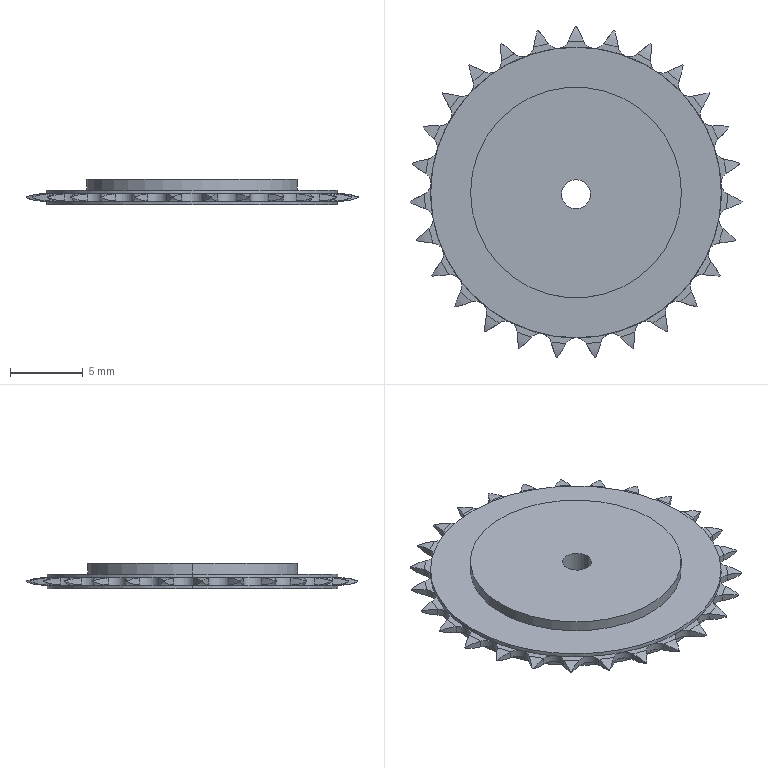Part | SolidWorks | features ICE 4, Scale 3, CirPattern 1, Extrusion 1 | 1 solid | 227 faces | box 22.854 x 22.815 x 1.75 mm | volume 447.235 mm3 | cylinder 143 | plane 84 | commonest cylinder face diameters 6.25 x54 22.214 x54 1.59 x27 20.001 x4 2 x2 14.516 x2